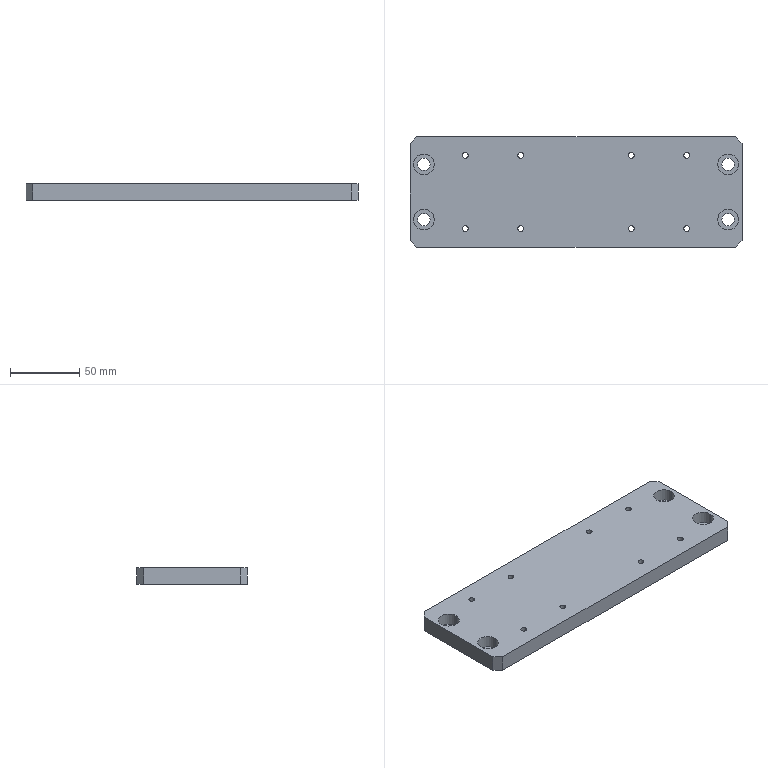Part | SolidWorks | features BaseBody 1 | 1 solid | 46 faces | box 240 x 80 x 12 mm | volume 221345 mm3 | cylinder 32 | plane 14 | commonest cylinder face diameters 4.2 x16 9 x8 15 x8
STEP:
#1=CARTESIAN_POINT('',(77.9,26.5,0.));
#2=VERTEX_POINT('',#1);
#3=CARTESIAN_POINT('',(82.1,26.5,0.));
#4=VERTEX_POINT('',#3);
#5=CARTESIAN_POINT('',(80.,26.5,0.));
#6=DIRECTION('',(0.,0.,1.));
#7=DIRECTION('',(1.,0.,0.));
#8=AXIS2_PLACEMENT_3D('',#5,#6,#7);
#9=CIRCLE('',#8,2.1);
#10=EDGE_CURVE('',#2,#4,#9,.T.);
#11=ORIENTED_EDGE('',*,*,#10,.F.);
#12=CARTESIAN_POINT('',(77.9,26.5,12.));
#13=VERTEX_POINT('',#12);
#14=CARTESIAN_POINT('',(77.9,26.5,12.));
#15=DIRECTION('',(0.,0.,1.));
#16=VECTOR('',#15,1000.);
#17=LINE('',#14,#16);
#18=EDGE_CURVE('',#2,#13,#17,.T.);
#19=ORIENTED_EDGE('',*,*,#18,.T.);
#20=CARTESIAN_POINT('',(82.1,26.5,12.));
#21=VERTEX_POINT('',#20);
#22=CARTESIAN_POINT('',(80.,26.5,12.));
#23=DIRECTION('',(0.,0.,-1.));
#24=DIRECTION('',(1.,0.,0.));
#25=AXIS2_PLACEMENT_3D('',#22,#23,#24);
#26=CIRCLE('',#25,2.1);
#27=EDGE_CURVE('',#21,#13,#26,.T.);
#28=ORIENTED_EDGE('',*,*,#27,.F.);
#29=CARTESIAN_POINT('',(82.1,26.5,12.));
#30=DIRECTION('',(0.,0.,1.));
#31=VECTOR('',#30,1000.);
#32=LINE('',#29,#31);
#33=EDGE_CURVE('',#4,#21,#32,.T.);
#34=ORIENTED_EDGE('',*,*,#33,.F.);
#35=EDGE_LOOP('',(#11,#19,#28,#34));
#36=FACE_OUTER_BOUND('',#35,.T.);
#37=CARTESIAN_POINT('',(80.,26.5,12.));
#38=DIRECTION('',(0.,0.,1.));
#39=DIRECTION('',(1.,0.,0.));
#40=AXIS2_PLACEMENT_3D('',#37,#38,#39);
#41=CYLINDRICAL_SURFACE('',#40,2.1);
#42=ADVANCED_FACE('',(#36),#41,.F.);
#43=CARTESIAN_POINT('',(77.9,-26.5,0.));
#44=VERTEX_POINT('',#43);
#45=CARTESIAN_POINT('',(82.1,-26.5,0.));
#46=VERTEX_POINT('',#45);
#47=CARTESIAN_POINT('',(80.,-26.5,0.));
#48=DIRECTION('',(0.,0.,1.));
#49=DIRECTION('',(1.,0.,0.));
#50=AXIS2_PLACEMENT_3D('',#47,#48,#49);
#51=CIRCLE('',#50,2.1);
#52=EDGE_CURVE('',#44,#46,#51,.T.);
#53=ORIENTED_EDGE('',*,*,#52,.F.);
#54=CARTESIAN_POINT('',(77.9,-26.5,12.));
#55=VERTEX_POINT('',#54);
#56=CARTESIAN_POINT('',(77.9,-26.5,12.));
#57=DIRECTION('',(0.,0.,1.));
#58=VECTOR('',#57,1000.);
#59=LINE('',#56,#58);
#60=EDGE_CURVE('',#44,#55,#59,.T.);
#61=ORIENTED_EDGE('',*,*,#60,.T.);
#62=CARTESIAN_POINT('',(82.1,-26.5,12.));
#63=VERTEX_POINT('',#62);
#64=CARTESIAN_POINT('',(80.,-26.5,12.));
#65=DIRECTION('',(0.,0.,-1.));
#66=DIRECTION('',(1.,0.,0.));
#67=AXIS2_PLACEMENT_3D('',#64,#65,#66);
#68=CIRCLE('',#67,2.1);
#69=EDGE_CURVE('',#63,#55,#68,.T.);
#70=ORIENTED_EDGE('',*,*,#69,.F.);
#71=CARTESIAN_POINT('',(82.1,-26.5,12.));
#72=DIRECTION('',(0.,0.,1.));
#73=VECTOR('',#72,1000.);
#74=LINE('',#71,#73);
#75=EDGE_CURVE('',#46,#63,#74,.T.);
#76=ORIENTED_EDGE('',*,*,#75,.F.);
#77=EDGE_LOOP('',(#53,#61,#70,#76));
#78=FACE_OUTER_BOUND('',#77,.T.);
#79=CARTESIAN_POINT('',(80.,-26.5,12.));
#80=DIRECTION('',(0.,0.,1.));
#81=DIRECTION('',(1.,0.,0.));
#82=AXIS2_PLACEMENT_3D('',#79,#80,#81);
#83=CYLINDRICAL_SURFACE('',#82,2.1);
#84=ADVANCED_FACE('',(#78),#83,.F.);
#85=CARTESIAN_POINT('',(37.9,-26.5,0.));
#86=VERTEX_POINT('',#85);
#87=CARTESIAN_POINT('',(42.1,-26.5,0.));
#88=VERTEX_POINT('',#87);
#89=CARTESIAN_POINT('',(40.,-26.5,0.));
#90=DIRECTION('',(0.,0.,1.));
#91=DIRECTION('',(1.,0.,0.));
#92=AXIS2_PLACEMENT_3D('',#89,#90,#91);
#93=CIRCLE('',#92,2.1);
#94=EDGE_CURVE('',#86,#88,#93,.T.);
#95=ORIENTED_EDGE('',*,*,#94,.F.);
#96=CARTESIAN_POINT('',(37.9,-26.5,12.));
#97=VERTEX_POINT('',#96);
#98=CARTESIAN_POINT('',(37.9,-26.5,12.));
#99=DIRECTION('',(0.,0.,1.));
#100=VECTOR('',#99,1000.);
#101=LINE('',#98,#100);
#102=EDGE_CURVE('',#86,#97,#101,.T.);
#103=ORIENTED_EDGE('',*,*,#102,.T.);
#104=CARTESIAN_POINT('',(42.1,-26.5,12.));
#105=VERTEX_POINT('',#104);
#106=CARTESIAN_POINT('',(40.,-26.5,12.));
#107=DIRECTION('',(0.,0.,-1.));
#108=DIRECTION('',(1.,0.,0.));
#109=AXIS2_PLACEMENT_3D('',#106,#107,#108);
#110=CIRCLE('',#109,2.1);
#111=EDGE_CURVE('',#105,#97,#110,.T.);
#112=ORIENTED_EDGE('',*,*,#111,.F.);
#113=CARTESIAN_POINT('',(42.1,-26.5,12.));
#114=DIRECTION('',(0.,0.,1.));
#115=VECTOR('',#114,1000.);
#116=LINE('',#113,#115);
#117=EDGE_CURVE('',#88,#105,#116,.T.);
#118=ORIENTED_EDGE('',*,*,#117,.F.);
#119=EDGE_LOOP('',(#95,#103,#112,#118));
#120=FACE_OUTER_BOUND('',#119,.T.);
#121=CARTESIAN_POINT('',(40.,-26.5,12.));
#122=DIRECTION('',(0.,0.,1.));
#123=DIRECTION('',(1.,0.,0.));
#124=AXIS2_PLACEMENT_3D('',#121,#122,#123);
#125=CYLINDRICAL_SURFACE('',#124,2.1);
#126=ADVANCED_FACE('',(#120),#125,.F.);
#127=CARTESIAN_POINT('',(37.9,26.5,0.));
#128=VERTEX_POINT('',#127);
#129=CARTESIAN_POINT('',(42.1,26.5,0.));
#130=VERTEX_POINT('',#129);
#131=CARTESIAN_POINT('',(40.,26.5,0.));
#132=DIRECTION('',(0.,0.,1.));
#133=DIRECTION('',(1.,0.,0.));
#134=AXIS2_PLACEMENT_3D('',#131,#132,#133);
#135=CIRCLE('',#134,2.1);
#136=EDGE_CURVE('',#128,#130,#135,.T.);
#137=ORIENTED_EDGE('',*,*,#136,.F.);
#138=CARTESIAN_POINT('',(37.9,26.5,12.));
#139=VERTEX_POINT('',#138);
#140=CARTESIAN_POINT('',(37.9,26.5,12.));
#141=DIRECTION('',(0.,0.,1.));
#142=VECTOR('',#141,1000.);
#143=LINE('',#140,#142);
#144=EDGE_CURVE('',#128,#139,#143,.T.);
#145=ORIENTED_EDGE('',*,*,#144,.T.);
#146=CARTESIAN_POINT('',(42.1,26.5,12.));
#147=VERTEX_POINT('',#146);
#148=CARTESIAN_POINT('',(40.,26.5,12.));
#149=DIRECTION('',(0.,0.,-1.));
#150=DIRECTION('',(1.,0.,0.));
#151=AXIS2_PLACEMENT_3D('',#148,#149,#150);
#152=CIRCLE('',#151,2.1);
#153=EDGE_CURVE('',#147,#139,#152,.T.);
#154=ORIENTED_EDGE('',*,*,#153,.F.);
#155=CARTESIAN_POINT('',(42.1,26.5,12.));
#156=DIRECTION('',(0.,0.,1.));
#157=VECTOR('',#156,1000.);
#158=LINE('',#155,#157);
#159=EDGE_CURVE('',#130,#147,#158,.T.);
#160=ORIENTED_EDGE('',*,*,#159,.F.);
#161=EDGE_LOOP('',(#137,#145,#154,#160));
#162=FACE_OUTER_BOUND('',#161,.T.);
#163=CARTESIAN_POINT('',(40.,26.5,12.));
#164=DIRECTION('',(0.,0.,1.));
#165=DIRECTION('',(1.,0.,0.));
#166=AXIS2_PLACEMENT_3D('',#163,#164,#165);
#167=CYLINDRICAL_SURFACE('',#166,2.1);
#168=ADVANCED_FACE('',(#162),#167,.F.);
#169=CARTESIAN_POINT('',(-42.1,26.5,0.));
#170=VERTEX_POINT('',#169);
#171=CARTESIAN_POINT('',(-37.9,26.5,0.));
#172=VERTEX_POINT('',#171);
#173=CARTESIAN_POINT('',(-40.,26.5,0.));
#174=DIRECTION('',(0.,0.,1.));
#175=DIRECTION('',(1.,0.,0.));
#176=AXIS2_PLACEMENT_3D('',#173,#174,#175);
#177=CIRCLE('',#176,2.1);
#178=EDGE_CURVE('',#170,#172,#177,.T.);
#179=ORIENTED_EDGE('',*,*,#178,.F.);
#180=CARTESIAN_POINT('',(-42.1,26.5,12.));
#181=VERTEX_POINT('',#180);
#182=CARTESIAN_POINT('',(-42.1,26.5,12.));
#183=DIRECTION('',(0.,0.,1.));
#184=VECTOR('',#183,1000.);
#185=LINE('',#182,#184);
#186=EDGE_CURVE('',#170,#181,#185,.T.);
#187=ORIENTED_EDGE('',*,*,#186,.T.);
#188=CARTESIAN_POINT('',(-37.9,26.5,12.));
#189=VERTEX_POINT('',#188);
#190=CARTESIAN_POINT('',(-40.,26.5,12.));
#191=DIRECTION('',(0.,0.,-1.));
#192=DIRECTION('',(1.,0.,0.));
#193=AXIS2_PLACEMENT_3D('',#190,#191,#192);
#194=CIRCLE('',#193,2.1);
#195=EDGE_CURVE('',#189,#181,#194,.T.);
#196=ORIENTED_EDGE('',*,*,#195,.F.);
#197=CARTESIAN_POINT('',(-37.9,26.5,12.));
#198=DIRECTION('',(0.,0.,1.));
#199=VECTOR('',#198,1000.);
#200=LINE('',#197,#199);
#201=EDGE_CURVE('',#172,#189,#200,.T.);
#202=ORIENTED_EDGE('',*,*,#201,.F.);
#203=EDGE_LOOP('',(#179,#187,#196,#202));
#204=FACE_OUTER_BOUND('',#203,.T.);
#205=CARTESIAN_POINT('',(-40.,26.5,12.));
#206=DIRECTION('',(0.,0.,1.));
#207=DIRECTION('',(1.,0.,0.));
#208=AXIS2_PLACEMENT_3D('',#205,#206,#207);
#209=CYLINDRICAL_SURFACE('',#208,2.1);
#210=ADVANCED_FACE('',(#204),#209,.F.);
#211=CARTESIAN_POINT('',(-42.1,-26.5,0.));
#212=VERTEX_POINT('',#211);
#213=CARTESIAN_POINT('',(-37.9,-26.5,0.));
#214=VERTEX_POINT('',#213);
#215=CARTESIAN_POINT('',(-40.,-26.5,0.));
#216=DIRECTION('',(0.,0.,1.));
#217=DIRECTION('',(1.,0.,0.));
#218=AXIS2_PLACEMENT_3D('',#215,#216,#217);
#219=CIRCLE('',#218,2.1);
#220=EDGE_CURVE('',#212,#214,#219,.T.);
#221=ORIENTED_EDGE('',*,*,#220,.F.);
#222=CARTESIAN_POINT('',(-42.1,-26.5,12.));
#223=VERTEX_POINT('',#222);
#224=CARTESIAN_POINT('',(-42.1,-26.5,12.));
#225=DIRECTION('',(0.,0.,1.));
#226=VECTOR('',#225,1000.);
#227=LINE('',#224,#226);
#228=EDGE_CURVE('',#212,#223,#227,.T.);
#229=ORIENTED_EDGE('',*,*,#228,.T.);
#230=CARTESIAN_POINT('',(-37.9,-26.5,12.));
#231=VERTEX_POINT('',#230);
#232=CARTESIAN_POINT('',(-40.,-26.5,12.));
#233=DIRECTION('',(0.,0.,-1.));
#234=DIRECTION('',(1.,0.,0.));
#235=AXIS2_PLACEMENT_3D('',#232,#233,#234);
#236=CIRCLE('',#235,2.1);
#237=EDGE_CURVE('',#231,#223,#236,.T.);
#238=ORIENTED_EDGE('',*,*,#237,.F.);
#239=CARTESIAN_POINT('',(-37.9,-26.5,12.));
#240=DIRECTION('',(0.,0.,1.));
#241=VECTOR('',#240,1000.);
#242=LINE('',#239,#241);
#243=EDGE_CURVE('',#214,#231,#242,.T.);
#244=ORIENTED_EDGE('',*,*,#243,.F.);
#245=EDGE_LOOP('',(#221,#229,#238,#244));
#246=FACE_OUTER_BOUND('',#245,.T.);
#247=CARTESIAN_POINT('',(-40.,-26.5,12.));
#248=DIRECTION('',(0.,0.,1.));
#249=DIRECTION('',(1.,0.,0.));
#250=AXIS2_PLACEMENT_3D('',#247,#248,#249);
#251=CYLINDRICAL_SURFACE('',#250,2.1);
#252=ADVANCED_FACE('',(#246),#251,.F.);
#253=CARTESIAN_POINT('',(-82.1,-26.5,0.));
#254=VERTEX_POINT('',#253);
#255=CARTESIAN_POINT('',(-77.9,-26.5,0.));
#256=VERTEX_POINT('',#255);
#257=CARTESIAN_POINT('',(-80.,-26.5,0.));
#258=DIRECTION('',(0.,0.,1.));
#259=DIRECTION('',(1.,0.,0.));
#260=AXIS2_PLACEMENT_3D('',#257,#258,#259);
#261=CIRCLE('',#260,2.1);
#262=EDGE_CURVE('',#254,#256,#261,.T.);
#263=ORIENTED_EDGE('',*,*,#262,.F.);
#264=CARTESIAN_POINT('',(-82.1,-26.5,12.));
#265=VERTEX_POINT('',#264);
#266=CARTESIAN_POINT('',(-82.1,-26.5,12.));
#267=DIRECTION('',(0.,0.,1.));
#268=VECTOR('',#267,1000.);
#269=LINE('',#266,#268);
#270=EDGE_CURVE('',#254,#265,#269,.T.);
#271=ORIENTED_EDGE('',*,*,#270,.T.);
#272=CARTESIAN_POINT('',(-77.9,-26.5,12.));
#273=VERTEX_POINT('',#272);
#274=CARTESIAN_POINT('',(-80.,-26.5,12.));
#275=DIRECTION('',(0.,0.,-1.));
#276=DIRECTION('',(1.,0.,0.));
#277=AXIS2_PLACEMENT_3D('',#274,#275,#276);
#278=CIRCLE('',#277,2.1);
#279=EDGE_CURVE('',#273,#265,#278,.T.);
#280=ORIENTED_EDGE('',*,*,#279,.F.);
#281=CARTESIAN_POINT('',(-77.9,-26.5,12.));
#282=DIRECTION('',(0.,0.,1.));
#283=VECTOR('',#282,1000.);
#284=LINE('',#281,#283);
#285=EDGE_CURVE('',#256,#273,#284,.T.);
#286=ORIENTED_EDGE('',*,*,#285,.F.);
#287=EDGE_LOOP('',(#263,#271,#280,#286));
#288=FACE_OUTER_BOUND('',#287,.T.);
#289=CARTESIAN_POINT('',(-80.,-26.5,12.));
#290=DIRECTION('',(0.,0.,1.));
#291=DIRECTION('',(1.,0.,0.));
#292=AXIS2_PLACEMENT_3D('',#289,#290,#291);
#293=CYLINDRICAL_SURFACE('',#292,2.1);
#294=ADVANCED_FACE('',(#288),#293,.F.);
#295=CARTESIAN_POINT('',(-82.1,26.5,0.));
#296=VERTEX_POINT('',#295);
#297=CARTESIAN_POINT('',(-77.9,26.5,0.));
#298=VERTEX_POINT('',#297);
#299=CARTESIAN_POINT('',(-80.,26.5,0.));
#300=DIRECTION('',(0.,0.,1.));
#301=DIRECTION('',(1.,0.,0.));
#302=AXIS2_PLACEMENT_3D('',#299,#300,#301);
#303=CIRCLE('',#302,2.1);
#304=EDGE_CURVE('',#296,#298,#303,.T.);
#305=ORIENTED_EDGE('',*,*,#304,.F.);
#306=CARTESIAN_POINT('',(-82.1,26.5,12.));
#307=VERTEX_POINT('',#306);
#308=CARTESIAN_POINT('',(-82.1,26.5,12.));
#309=DIRECTION('',(0.,0.,1.));
#310=VECTOR('',#309,1000.);
#311=LINE('',#308,#310);
#312=EDGE_CURVE('',#296,#307,#311,.T.);
#313=ORIENTED_EDGE('',*,*,#312,.T.);
#314=CARTESIAN_POINT('',(-77.9,26.5,12.));
#315=VERTEX_POINT('',#314);
#316=CARTESIAN_POINT('',(-80.,26.5,12.));
#317=DIRECTION('',(0.,0.,-1.));
#318=DIRECTION('',(1.,0.,0.));
#319=AXIS2_PLACEMENT_3D('',#316,#317,#318);
#320=CIRCLE('',#319,2.1);
#321=EDGE_CURVE('',#315,#307,#320,.T.);
#322=ORIENTED_EDGE('',*,*,#321,.F.);
#323=CARTESIAN_POINT('',(-77.9,26.5,12.));
#324=DIRECTION('',(0.,0.,1.));
#325=VECTOR('',#324,1000.);
#326=LINE('',#323,#325);
#327=EDGE_CURVE('',#298,#315,#326,.T.);
#328=ORIENTED_EDGE('',*,*,#327,.F.);
#329=EDGE_LOOP('',(#305,#313,#322,#328));
#330=FACE_OUTER_BOUND('',#329,.T.);
#331=CARTESIAN_POINT('',(-80.,26.5,12.));
#332=DIRECTION('',(0.,0.,1.));
#333=DIRECTION('',(1.,0.,0.));
#334=AXIS2_PLACEMENT_3D('',#331,#332,#333);
#335=CYLINDRICAL_SURFACE('',#334,2.1);
#336=ADVANCED_FACE('',(#330),#335,.F.);
#337=CARTESIAN_POINT('',(105.5,20.,0.));
#338=VERTEX_POINT('',#337);
#339=CARTESIAN_POINT('',(114.5,20.,0.));
#340=VERTEX_POINT('',#339);
#341=CARTESIAN_POINT('',(110.,20.,0.));
#342=DIRECTION('',(0.,0.,1.));
#343=DIRECTION('',(1.,0.,0.));
#344=AXIS2_PLACEMENT_3D('',#341,#342,#343);
#345=CIRCLE('',#344,4.5);
#346=EDGE_CURVE('',#338,#340,#345,.T.);
#347=ORIENTED_EDGE('',*,*,#346,.F.);
#348=CARTESIAN_POINT('',(105.5,20.,3.));
#349=VERTEX_POINT('',#348);
#350=CARTESIAN_POINT('',(105.5,20.,12.));
#351=DIRECTION('',(0.,0.,1.));
#352=VECTOR('',#351,1000.);
#353=LINE('',#350,#352);
#354=EDGE_CURVE('',#338,#349,#353,.T.);
#355=ORIENTED_EDGE('',*,*,#354,.T.);
#356=CARTESIAN_POINT('',(114.5,20.,3.));
#357=VERTEX_POINT('',#356);
#358=CARTESIAN_POINT('',(110.,20.,3.));
#359=DIRECTION('',(0.,0.,-1.));
#360=DIRECTION('',(1.,0.,0.));
#361=AXIS2_PLACEMENT_3D('',#358,#359,#360);
#362=CIRCLE('',#361,4.5);
#363=EDGE_CURVE('',#357,#349,#362,.T.);
#364=ORIENTED_EDGE('',*,*,#363,.F.);
#365=CARTESIAN_POINT('',(114.5,20.,12.));
#366=DIRECTION('',(0.,0.,1.));
#367=VECTOR('',#366,1000.);
#368=LINE('',#365,#367);
#369=EDGE_CURVE('',#340,#357,#368,.T.);
#370=ORIENTED_EDGE('',*,*,#369,.F.);
#371=EDGE_LOOP('',(#347,#355,#364,#370));
#372=FACE_OUTER_BOUND('',#371,.T.);
#373=CARTESIAN_POINT('',(110.,20.,12.));
#374=DIRECTION('',(0.,0.,1.));
#375=DIRECTION('',(1.,0.,0.));
#376=AXIS2_PLACEMENT_3D('',#373,#374,#375);
#377=CYLINDRICAL_SURFACE('',#376,4.5);
#378=ADVANCED_FACE('',(#372),#377,.F.);
#379=CARTESIAN_POINT('',(105.5,-20.,0.));
#380=VERTEX_POINT('',#379);
#381=CARTESIAN_POINT('',(114.5,-20.,0.));
#382=VERTEX_POINT('',#381);
#383=CARTESIAN_POINT('',(110.,-20.,0.));
#384=DIRECTION('',(0.,0.,1.));
#385=DIRECTION('',(1.,0.,0.));
#386=AXIS2_PLACEMENT_3D('',#383,#384,#385);
#387=CIRCLE('',#386,4.5);
#388=EDGE_CURVE('',#380,#382,#387,.T.);
#389=ORIENTED_EDGE('',*,*,#388,.F.);
#390=CARTESIAN_POINT('',(105.5,-20.,3.));
#391=VERTEX_POINT('',#390);
#392=CARTESIAN_POINT('',(105.5,-20.,12.));
#393=DIRECTION('',(0.,0.,1.));
#394=VECTOR('',#393,1000.);
#395=LINE('',#392,#394);
#396=EDGE_CURVE('',#380,#391,#395,.T.);
#397=ORIENTED_EDGE('',*,*,#396,.T.);
#398=CARTESIAN_POINT('',(114.5,-20.,3.));
#399=VERTEX_POINT('',#398);
#400=CARTESIAN_POINT('',(110.,-20.,3.));
#401=DIRECTION('',(0.,0.,-1.));
#402=DIRECTION('',(1.,0.,0.));
#403=AXIS2_PLACEMENT_3D('',#400,#401,#402);
#404=CIRCLE('',#403,4.5);
#405=EDGE_CURVE('',#399,#391,#404,.T.);
#406=ORIENTED_EDGE('',*,*,#405,.F.);
#407=CARTESIAN_POINT('',(114.5,-20.,12.));
#408=DIRECTION('',(0.,0.,1.));
#409=VECTOR('',#408,1000.);
#410=LINE('',#407,#409);
#411=EDGE_CURVE('',#382,#399,#410,.T.);
#412=ORIENTED_EDGE('',*,*,#411,.F.);
#413=EDGE_LOOP('',(#389,#397,#406,#412));
#414=FACE_OUTER_BOUND('',#413,.T.);
#415=CARTESIAN_POINT('',(110.,-20.,12.));
#416=DIRECTION('',(0.,0.,1.));
#417=DIRECTION('',(1.,0.,0.));
#418=AXIS2_PLACEMENT_3D('',#415,#416,#417);
#419=CYLINDRICAL_SURFACE('',#418,4.5);
#420=ADVANCED_FACE('',(#414),#419,.F.);
#421=CARTESIAN_POINT('',(-114.5,-20.,0.));
#422=VERTEX_POINT('',#421);
#423=CARTESIAN_POINT('',(-105.5,-20.,0.));
#424=VERTEX_POINT('',#423);
#425=CARTESIAN_POINT('',(-110.,-20.,0.));
#426=DIRECTION('',(0.,0.,1.));
#427=DIRECTION('',(1.,0.,0.));
#428=AXIS2_PLACEMENT_3D('',#425,#426,#427);
#429=CIRCLE('',#428,4.5);
#430=EDGE_CURVE('',#422,#424,#429,.T.);
#431=ORIENTED_EDGE('',*,*,#430,.F.);
#432=CARTESIAN_POINT('',(-114.5,-20.,3.));
#433=VERTEX_POINT('',#432);
#434=CARTESIAN_POINT('',(-114.5,-20.,12.));
#435=DIRECTION('',(0.,0.,1.));
#436=VECTOR('',#435,1000.);
#437=LINE('',#434,#436);
#438=EDGE_CURVE('',#422,#433,#437,.T.);
#439=ORIENTED_EDGE('',*,*,#438,.T.);
#440=CARTESIAN_POINT('',(-105.5,-20.,3.));
#441=VERTEX_POINT('',#440);
#442=CARTESIAN_POINT('',(-110.,-20.,3.));
#443=DIRECTION('',(0.,0.,-1.));
#444=DIRECTION('',(1.,0.,0.));
#445=AXIS2_PLACEMENT_3D('',#442,#443,#444);
#446=CIRCLE('',#445,4.5);
#447=EDGE_CURVE('',#441,#433,#446,.T.);
#448=ORIENTED_EDGE('',*,*,#447,.F.);
#449=CARTESIAN_POINT('',(-105.5,-20.,12.));
#450=DIRECTION('',(0.,0.,1.));
#451=VECTOR('',#450,1000.);
#452=LINE('',#449,#451);
#453=EDGE_CURVE('',#424,#441,#452,.T.);
#454=ORIENTED_EDGE('',*,*,#453,.F.);
#455=EDGE_LOOP('',(#431,#439,#448,#454));
#456=FACE_OUTER_BOUND('',#455,.T.);
#457=CARTESIAN_POINT('',(-110.,-20.,12.));
#458=DIRECTION('',(0.,0.,1.));
#459=DIRECTION('',(1.,0.,0.));
#460=AXIS2_PLACEMENT_3D('',#457,#458,#459);
#461=CYLINDRICAL_SURFACE('',#460,4.5);
#462=ADVANCED_FACE('',(#456),#461,.F.);
#463=CARTESIAN_POINT('',(-114.5,20.,0.));
#464=VERTEX_POINT('',#463);
#465=CARTESIAN_POINT('',(-105.5,20.,0.));
#466=VERTEX_POINT('',#465);
#467=CARTESIAN_POINT('',(-110.,20.,0.));
#468=DIRECTION('',(0.,0.,1.));
#469=DIRECTION('',(1.,0.,0.));
#470=AXIS2_PLACEMENT_3D('',#467,#468,#469);
#471=CIRCLE('',#470,4.5);
#472=EDGE_CURVE('',#464,#466,#471,.T.);
#473=ORIENTED_EDGE('',*,*,#472,.F.);
#474=CARTESIAN_POINT('',(-114.5,20.,3.));
#475=VERTEX_POINT('',#474);
#476=CARTESIAN_POINT('',(-114.5,20.,12.));
#477=DIRECTION('',(0.,0.,1.));
#478=VECTOR('',#477,1000.);
#479=LINE('',#476,#478);
#480=EDGE_CURVE('',#464,#475,#479,.T.);
#481=ORIENTED_EDGE('',*,*,#480,.T.);
#482=CARTESIAN_POINT('',(-105.5,20.,3.));
#483=VERTEX_POINT('',#482);
#484=CARTESIAN_POINT('',(-110.,20.,3.));
#485=DIRECTION('',(0.,0.,-1.));
#486=DIRECTION('',(1.,0.,0.));
#487=AXIS2_PLACEMENT_3D('',#484,#485,#486);
#488=CIRCLE('',#487,4.5);
#489=EDGE_CURVE('',#483,#475,#488,.T.);
#490=ORIENTED_EDGE('',*,*,#489,.F.);
#491=CARTESIAN_POINT('',(-105.5,20.,12.));
#492=DIRECTION('',(0.,0.,1.));
#493=VECTOR('',#492,1000.);
#494=LINE('',#491,#493);
#495=EDGE_CURVE('',#466,#483,#494,.T.);
#496=ORIENTED_EDGE('',*,*,#495,.F.);
#497=EDGE_LOOP('',(#473,#481,#490,#496));
#498=FACE_OUTER_BOUND('',#497,.T.);
#499=CARTESIAN_POINT('',(-110.,20.,12.));
#500=DIRECTION('',(0.,0.,1.));
#501=DIRECTION('',(1.,0.,0.));
#502=AXIS2_PLACEMENT_3D('',#499,#500,#501);
#503=CYLINDRICAL_SURFACE('',#502,4.5);
#504=ADVANCED_FACE('',(#498),#503,.F.);
#505=CARTESIAN_POINT('',(-102.5,-20.,3.));
#506=VERTEX_POINT('',#505);
#507=CARTESIAN_POINT('',(-117.5,-20.,3.));
#508=VERTEX_POINT('',#507);
#509=CARTESIAN_POINT('',(-110.,-20.,3.));
#510=DIRECTION('',(0.,0.,-1.));
#511=DIRECTION('',(1.,0.,0.));
#512=AXIS2_PLACEMENT_3D('',#509,#510,#511);
#513=CIRCLE('',#512,7.5);
#514=EDGE_CURVE('',#506,#508,#513,.T.);
#515=ORIENTED_EDGE('',*,*,#514,.T.);
#516=CARTESIAN_POINT('',(-117.5,-20.,12.));
#517=VERTEX_POINT('',#516);
#518=CARTESIAN_POINT('',(-117.5,-20.,12.));
#519=DIRECTION('',(0.,0.,1.));
#520=VECTOR('',#519,1000.);
#521=LINE('',#518,#520);
#522=EDGE_CURVE('',#508,#517,#521,.T.);
#523=ORIENTED_EDGE('',*,*,#522,.T.);
#524=CARTESIAN_POINT('',(-102.5,-20.,12.));
#525=VERTEX_POINT('',#524);
#526=CARTESIAN_POINT('',(-110.,-20.,12.));
#527=DIRECTION('',(0.,0.,1.));
#528=DIRECTION('',(1.,0.,0.));
#529=AXIS2_PLACEMENT_3D('',#526,#527,#528);
#530=CIRCLE('',#529,7.5);
#531=EDGE_CURVE('',#517,#525,#530,.T.);
#532=ORIENTED_EDGE('',*,*,#531,.T.);
#533=CARTESIAN_POINT('',(-102.5,-20.,12.));
#534=DIRECTION('',(0.,0.,1.));
#535=VECTOR('',#534,1000.);
#536=LINE('',#533,#535);
#537=EDGE_CURVE('',#506,#525,#536,.T.);
#538=ORIENTED_EDGE('',*,*,#537,.F.);
#539=EDGE_LOOP('',(#515,#523,#532,#538));
#540=FACE_OUTER_BOUND('',#539,.T.);
#541=CARTESIAN_POINT('',(-110.,-20.,12.));
#542=DIRECTION('',(0.,0.,1.));
#543=DIRECTION('',(1.,0.,0.));
#544=AXIS2_PLACEMENT_3D('',#541,#542,#543);
#545=CYLINDRICAL_SURFACE('',#544,7.5);
#546=ADVANCED_FACE('',(#540),#545,.F.);
#547=CARTESIAN_POINT('',(117.5,-20.,3.));
#548=VERTEX_POINT('',#547);
#549=CARTESIAN_POINT('',(102.5,-20.,3.));
#550=VERTEX_POINT('',#549);
#551=CARTESIAN_POINT('',(110.,-20.,3.));
#552=DIRECTION('',(0.,0.,-1.));
#553=DIRECTION('',(1.,0.,0.));
#554=AXIS2_PLACEMENT_3D('',#551,#552,#553);
#555=CIRCLE('',#554,7.5);
#556=EDGE_CURVE('',#548,#550,#555,.T.);
#557=ORIENTED_EDGE('',*,*,#556,.T.);
#558=CARTESIAN_POINT('',(102.5,-20.,12.));
#559=VERTEX_POINT('',#558);
#560=CARTESIAN_POINT('',(102.5,-20.,12.));
#561=DIRECTION('',(0.,0.,1.));
#562=VECTOR('',#561,1000.);
#563=LINE('',#560,#562);
#564=EDGE_CURVE('',#550,#559,#563,.T.);
#565=ORIENTED_EDGE('',*,*,#564,.T.);
#566=CARTESIAN_POINT('',(117.5,-20.,12.));
#567=VERTEX_POINT('',#566);
#568=CARTESIAN_POINT('',(110.,-20.,12.));
#569=DIRECTION('',(0.,0.,1.));
#570=DIRECTION('',(1.,0.,0.));
#571=AXIS2_PLACEMENT_3D('',#568,#569,#570);
#572=CIRCLE('',#571,7.5);
#573=EDGE_CURVE('',#559,#567,#572,.T.);
#574=ORIENTED_EDGE('',*,*,#573,.T.);
#575=CARTESIAN_POINT('',(117.5,-20.,12.));
#576=DIRECTION('',(0.,0.,1.));
#577=VECTOR('',#576,1000.);
#578=LINE('',#575,#577);
#579=EDGE_CURVE('',#548,#567,#578,.T.);
#580=ORIENTED_EDGE('',*,*,#579,.F.);
#581=EDGE_LOOP('',(#557,#565,#574,#580));
#582=FACE_OUTER_BOUND('',#581,.T.);
#583=CARTESIAN_POINT('',(110.,-20.,12.));
#584=DIRECTION('',(0.,0.,1.));
#585=DIRECTION('',(1.,0.,0.));
#586=AXIS2_PLACEMENT_3D('',#583,#584,#585);
#587=CYLINDRICAL_SURFACE('',#586,7.5);
#588=ADVANCED_FACE('',(#582),#587,.F.);
#589=CARTESIAN_POINT('',(117.5,20.,3.));
#590=VERTEX_POINT('',#589);
#591=CARTESIAN_POINT('',(102.5,20.,3.));
#592=VERTEX_POINT('',#591);
#593=CARTESIAN_POINT('',(110.,20.,3.));
#594=DIRECTION('',(0.,0.,-1.));
#595=DIRECTION('',(1.,0.,0.));
#596=AXIS2_PLACEMENT_3D('',#593,#594,#595);
#597=CIRCLE('',#596,7.5);
#598=EDGE_CURVE('',#590,#592,#597,.T.);
#599=ORIENTED_EDGE('',*,*,#598,.T.);
#600=CARTESIAN_POINT('',(102.5,20.,12.));
#601=VERTEX_POINT('',#600);
#602=CARTESIAN_POINT('',(102.5,20.,12.));
#603=DIRECTION('',(0.,0.,1.));
#604=VECTOR('',#603,1000.);
#605=LINE('',#602,#604);
#606=EDGE_CURVE('',#592,#601,#605,.T.);
#607=ORIENTED_EDGE('',*,*,#606,.T.);
#608=CARTESIAN_POINT('',(117.5,20.,12.));
#609=VERTEX_POINT('',#608);
#610=CARTESIAN_POINT('',(110.,20.,12.));
#611=DIRECTION('',(0.,0.,1.));
#612=DIRECTION('',(1.,0.,0.));
#613=AXIS2_PLACEMENT_3D('',#610,#611,#612);
#614=CIRCLE('',#613,7.5);
#615=EDGE_CURVE('',#601,#609,#614,.T.);
#616=ORIENTED_EDGE('',*,*,#615,.T.);
#617=CARTESIAN_POINT('',(117.5,20.,12.));
#618=DIRECTION('',(0.,0.,1.));
#619=VECTOR('',#618,1000.);
#620=LINE('',#617,#619);
#621=EDGE_CURVE('',#590,#609,#620,.T.);
#622=ORIENTED_EDGE('',*,*,#621,.F.);
#623=EDGE_LOOP('',(#599,#607,#616,#622));
#624=FACE_OUTER_BOUND('',#623,.T.);
#625=CARTESIAN_POINT('',(110.,20.,12.));
#626=DIRECTION('',(0.,0.,1.));
#627=DIRECTION('',(1.,0.,0.));
#628=AXIS2_PLACEMENT_3D('',#625,#626,#627);
#629=CYLINDRICAL_SURFACE('',#628,7.5);
#630=ADVANCED_FACE('',(#624),#629,.F.);
#631=CARTESIAN_POINT('',(-102.5,20.,3.));
#632=VERTEX_POINT('',#631);
#633=CARTESIAN_POINT('',(-117.5,20.,3.));
#634=VERTEX_POINT('',#633);
#635=CARTESIAN_POINT('',(-110.,20.,3.));
#636=DIRECTION('',(0.,0.,-1.));
#637=DIRECTION('',(1.,0.,0.));
#638=AXIS2_PLACEMENT_3D('',#635,#636,#637);
#639=CIRCLE('',#638,7.5);
#640=EDGE_CURVE('',#632,#634,#639,.T.);
#641=ORIENTED_EDGE('',*,*,#640,.T.);
#642=CARTESIAN_POINT('',(-117.5,20.,12.));
#643=VERTEX_POINT('',#642);
#644=CARTESIAN_POINT('',(-117.5,20.,12.));
#645=DIRECTION('',(0.,0.,1.));
#646=VECTOR('',#645,1000.);
#647=LINE('',#644,#646);
#648=EDGE_CURVE('',#634,#643,#647,.T.);
#649=ORIENTED_EDGE('',*,*,#648,.T.);
#650=CARTESIAN_POINT('',(-102.5,20.,12.));
#651=VERTEX_POINT('',#650);
#652=CARTESIAN_POINT('',(-110.,20.,12.));
#653=DIRECTION('',(0.,0.,1.));
#654=DIRECTION('',(1.,0.,0.));
#655=AXIS2_PLACEMENT_3D('',#652,#653,#654);
#656=CIRCLE('',#655,7.5);
#657=EDGE_CURVE('',#643,#651,#656,.T.);
#658=ORIENTED_EDGE('',*,*,#657,.T.);
#659=CARTESIAN_POINT('',(-102.5,20.,12.));
#660=DIRECTION('',(0.,0.,1.));
#661=VECTOR('',#660,1000.);
#662=LINE('',#659,#661);
#663=EDGE_CURVE('',#632,#651,#662,.T.);
#664=ORIENTED_EDGE('',*,*,#663,.F.);
#665=EDGE_LOOP('',(#641,#649,#658,#664));
#666=FACE_OUTER_BOUND('',#665,.T.);
#667=CARTESIAN_POINT('',(-110.,20.,12.));
#668=DIRECTION('',(0.,0.,1.));
#669=DIRECTION('',(1.,0.,0.));
#670=AXIS2_PLACEMENT_3D('',#667,#668,#669);
#671=CYLINDRICAL_SURFACE('',#670,7.5);
#672=ADVANCED_FACE('',(#666),#671,.F.);
#673=CARTESIAN_POINT('',(-120.,-35.,0.));
#674=VERTEX_POINT('',#673);
#675=CARTESIAN_POINT('',(-120.,35.,0.));
#676=VERTEX_POINT('',#675);
#677=CARTESIAN_POINT('',(-120.,0.,0.));
#678=DIRECTION('',(0.,1.,0.));
#679=VECTOR('',#678,1000.);
#680=LINE('',#677,#679);
#681=EDGE_CURVE('',#674,#676,#680,.T.);
#682=ORIENTED_EDGE('',*,*,#681,.T.);
#683=CARTESIAN_POINT('',(-115.,40.,0.));
#684=VERTEX_POINT('',#683);
#685=CARTESIAN_POINT('',(-120.,35.,0.));
#686=DIRECTION('',(0.7071,0.7071,0.));
#687=VECTOR('',#686,1000.);
#688=LINE('',#685,#687);
#689=EDGE_CURVE('',#676,#684,#688,.T.);
#690=ORIENTED_EDGE('',*,*,#689,.T.);
#691=CARTESIAN_POINT('',(115.,40.,0.));
#692=VERTEX_POINT('',#691);
#693=CARTESIAN_POINT('',(0.,40.,0.));
#694=DIRECTION('',(1.,0.,0.));
#695=VECTOR('',#694,1000.);
#696=LINE('',#693,#695);
#697=EDGE_CURVE('',#684,#692,#696,.T.);
#698=ORIENTED_EDGE('',*,*,#697,.T.);
#699=CARTESIAN_POINT('',(120.,35.,0.));
#700=VERTEX_POINT('',#699);
#701=CARTESIAN_POINT('',(115.,40.,0.));
#702=DIRECTION('',(0.7071,-0.7071,0.));
#703=VECTOR('',#702,1000.);
#704=LINE('',#701,#703);
#705=EDGE_CURVE('',#692,#700,#704,.T.);
#706=ORIENTED_EDGE('',*,*,#705,.T.);
#707=CARTESIAN_POINT('',(120.,-35.,0.));
#708=VERTEX_POINT('',#707);
#709=CARTESIAN_POINT('',(120.,0.,0.));
#710=DIRECTION('',(0.,-1.,0.));
#711=VECTOR('',#710,1000.);
#712=LINE('',#709,#711);
#713=EDGE_CURVE('',#700,#708,#712,.T.);
#714=ORIENTED_EDGE('',*,*,#713,.T.);
#715=CARTESIAN_POINT('',(115.,-40.,0.));
#716=VERTEX_POINT('',#715);
#717=CARTESIAN_POINT('',(120.,-35.,0.));
#718=DIRECTION('',(-0.7071,-0.7071,0.));
#719=VECTOR('',#718,1000.);
#720=LINE('',#717,#719);
#721=EDGE_CURVE('',#708,#716,#720,.T.);
#722=ORIENTED_EDGE('',*,*,#721,.T.);
#723=CARTESIAN_POINT('',(-115.,-40.,0.));
#724=VERTEX_POINT('',#723);
#725=CARTESIAN_POINT('',(0.,-40.,0.));
#726=DIRECTION('',(-1.,0.,0.));
#727=VECTOR('',#726,1000.);
#728=LINE('',#725,#727);
#729=EDGE_CURVE('',#716,#724,#728,.T.);
#730=ORIENTED_EDGE('',*,*,#729,.T.);
#731=CARTESIAN_POINT('',(-115.,-40.,0.));
#732=DIRECTION('',(-0.7071,0.7071,0.));
#733=VECTOR('',#732,1000.);
#734=LINE('',#731,#733);
#735=EDGE_CURVE('',#724,#674,#734,.T.);
#736=ORIENTED_EDGE('',*,*,#735,.T.);
#737=EDGE_LOOP('',(#682,#690,#698,#706,#714,#722,#730,#736));
#738=FACE_OUTER_BOUND('',#737,.T.);
#739=CARTESIAN_POINT('',(80.,26.5,0.));
#740=DIRECTION('',(0.,0.,1.));
#741=DIRECTION('',(1.,0.,0.));
#742=AXIS2_PLACEMENT_3D('',#739,#740,#741);
#743=CIRCLE('',#742,2.1);
#744=EDGE_CURVE('',#4,#2,#743,.T.);
#745=ORIENTED_EDGE('',*,*,#744,.T.);
#746=ORIENTED_EDGE('',*,*,#10,.T.);
#747=EDGE_LOOP('',(#745,#746));
#748=FACE_BOUND('',#747,.T.);
#749=CARTESIAN_POINT('',(80.,-26.5,0.));
#750=DIRECTION('',(0.,0.,1.));
#751=DIRECTION('',(1.,0.,0.));
#752=AXIS2_PLACEMENT_3D('',#749,#750,#751);
#753=CIRCLE('',#752,2.1);
#754=EDGE_CURVE('',#46,#44,#753,.T.);
#755=ORIENTED_EDGE('',*,*,#754,.T.);
#756=ORIENTED_EDGE('',*,*,#52,.T.);
#757=EDGE_LOOP('',(#755,#756));
#758=FACE_BOUND('',#757,.T.);
#759=CARTESIAN_POINT('',(40.,-26.5,0.));
#760=DIRECTION('',(0.,0.,1.));
#761=DIRECTION('',(1.,0.,0.));
#762=AXIS2_PLACEMENT_3D('',#759,#760,#761);
#763=CIRCLE('',#762,2.1);
#764=EDGE_CURVE('',#88,#86,#763,.T.);
#765=ORIENTED_EDGE('',*,*,#764,.T.);
#766=ORIENTED_EDGE('',*,*,#94,.T.);
#767=EDGE_LOOP('',(#765,#766));
#768=FACE_BOUND('',#767,.T.);
#769=CARTESIAN_POINT('',(40.,26.5,0.));
#770=DIRECTION('',(0.,0.,1.));
#771=DIRECTION('',(1.,0.,0.));
#772=AXIS2_PLACEMENT_3D('',#769,#770,#771);
#773=CIRCLE('',#772,2.1);
#774=EDGE_CURVE('',#130,#128,#773,.T.);
#775=ORIENTED_EDGE('',*,*,#774,.T.);
#776=ORIENTED_EDGE('',*,*,#136,.T.);
#777=EDGE_LOOP('',(#775,#776));
#778=FACE_BOUND('',#777,.T.);
#779=CARTESIAN_POINT('',(-40.,26.5,0.));
#780=DIRECTION('',(0.,0.,1.));
#781=DIRECTION('',(1.,0.,0.));
#782=AXIS2_PLACEMENT_3D('',#779,#780,#781);
#783=CIRCLE('',#782,2.1);
#784=EDGE_CURVE('',#172,#170,#783,.T.);
#785=ORIENTED_EDGE('',*,*,#784,.T.);
#786=ORIENTED_EDGE('',*,*,#178,.T.);
#787=EDGE_LOOP('',(#785,#786));
#788=FACE_BOUND('',#787,.T.);
#789=CARTESIAN_POINT('',(-40.,-26.5,0.));
#790=DIRECTION('',(0.,0.,1.));
#791=DIRECTION('',(1.,0.,0.));
#792=AXIS2_PLACEMENT_3D('',#789,#790,#791);
#793=CIRCLE('',#792,2.1);
#794=EDGE_CURVE('',#214,#212,#793,.T.);
#795=ORIENTED_EDGE('',*,*,#794,.T.);
#796=ORIENTED_EDGE('',*,*,#220,.T.);
#797=EDGE_LOOP('',(#795,#796));
#798=FACE_BOUND('',#797,.T.);
#799=CARTESIAN_POINT('',(-80.,-26.5,0.));
#800=DIRECTION('',(0.,0.,1.));
#801=DIRECTION('',(1.,0.,0.));
#802=AXIS2_PLACEMENT_3D('',#799,#800,#801);
#803=CIRCLE('',#802,2.1);
#804=EDGE_CURVE('',#256,#254,#803,.T.);
#805=ORIENTED_EDGE('',*,*,#804,.T.);
#806=ORIENTED_EDGE('',*,*,#262,.T.);
#807=EDGE_LOOP('',(#805,#806));
#808=FACE_BOUND('',#807,.T.);
#809=CARTESIAN_POINT('',(-80.,26.5,0.));
#810=DIRECTION('',(0.,0.,1.));
#811=DIRECTION('',(1.,0.,0.));
#812=AXIS2_PLACEMENT_3D('',#809,#810,#811);
#813=CIRCLE('',#812,2.1);
#814=EDGE_CURVE('',#298,#296,#813,.T.);
#815=ORIENTED_EDGE('',*,*,#814,.T.);
#816=ORIENTED_EDGE('',*,*,#304,.T.);
#817=EDGE_LOOP('',(#815,#816));
#818=FACE_BOUND('',#817,.T.);
#819=CARTESIAN_POINT('',(110.,20.,0.));
#820=DIRECTION('',(0.,0.,1.));
#821=DIRECTION('',(1.,0.,0.));
#822=AXIS2_PLACEMENT_3D('',#819,#820,#821);
#823=CIRCLE('',#822,4.5);
#824=EDGE_CURVE('',#340,#338,#823,.T.);
#825=ORIENTED_EDGE('',*,*,#824,.T.);
#826=ORIENTED_EDGE('',*,*,#346,.T.);
#827=EDGE_LOOP('',(#825,#826));
#828=FACE_BOUND('',#827,.T.);
#829=CARTESIAN_POINT('',(110.,-20.,0.));
#830=DIRECTION('',(0.,0.,1.));
#831=DIRECTION('',(1.,0.,0.));
#832=AXIS2_PLACEMENT_3D('',#829,#830,#831);
#833=CIRCLE('',#832,4.5);
#834=EDGE_CURVE('',#382,#380,#833,.T.);
#835=ORIENTED_EDGE('',*,*,#834,.T.);
#836=ORIENTED_EDGE('',*,*,#388,.T.);
#837=EDGE_LOOP('',(#835,#836));
#838=FACE_BOUND('',#837,.T.);
#839=CARTESIAN_POINT('',(-110.,-20.,0.));
#840=DIRECTION('',(0.,0.,1.));
#841=DIRECTION('',(1.,0.,0.));
#842=AXIS2_PLACEMENT_3D('',#839,#840,#841);
#843=CIRCLE('',#842,4.5);
#844=EDGE_CURVE('',#424,#422,#843,.T.);
#845=ORIENTED_EDGE('',*,*,#844,.T.);
#846=ORIENTED_EDGE('',*,*,#430,.T.);
#847=EDGE_LOOP('',(#845,#846));
#848=FACE_BOUND('',#847,.T.);
#849=CARTESIAN_POINT('',(-110.,20.,0.));
#850=DIRECTION('',(0.,0.,1.));
#851=DIRECTION('',(1.,0.,0.));
#852=AXIS2_PLACEMENT_3D('',#849,#850,#851);
#853=CIRCLE('',#852,4.5);
#854=EDGE_CURVE('',#466,#464,#853,.T.);
#855=ORIENTED_EDGE('',*,*,#854,.T.);
#856=ORIENTED_EDGE('',*,*,#472,.T.);
#857=EDGE_LOOP('',(#855,#856));
#858=FACE_BOUND('',#857,.T.);
#859=CARTESIAN_POINT('',(0.,0.,0.));
#860=DIRECTION('',(0.,0.,-1.));
#861=DIRECTION('',(-1.,0.,0.));
#862=AXIS2_PLACEMENT_3D('',#859,#860,#861);
#863=PLANE('',#862);
#864=ADVANCED_FACE('',(#738,#748,#758,#768,#778,#788,#798,#808,#818,#828,#838,#848,#858),#863,.T.);
#865=CARTESIAN_POINT('',(-115.,40.,12.));
#866=VERTEX_POINT('',#865);
#867=CARTESIAN_POINT('',(-115.,40.,12.));
#868=DIRECTION('',(0.,0.,1.));
#869=VECTOR('',#868,1000.);
#870=LINE('',#867,#869);
#871=EDGE_CURVE('',#684,#866,#870,.T.);
#872=ORIENTED_EDGE('',*,*,#871,.F.);
#873=ORIENTED_EDGE('',*,*,#689,.F.);
#874=CARTESIAN_POINT('',(-120.,35.,12.));
#875=VERTEX_POINT('',#874);
#876=CARTESIAN_POINT('',(-120.,35.,12.));
#877=DIRECTION('',(0.,0.,-1.));
#878=VECTOR('',#877,1000.);
#879=LINE('',#876,#878);
#880=EDGE_CURVE('',#875,#676,#879,.T.);
#881=ORIENTED_EDGE('',*,*,#880,.F.);
#882=CARTESIAN_POINT('',(-120.,35.,12.));
#883=DIRECTION('',(-0.7071,-0.7071,0.));
#884=VECTOR('',#883,1000.);
#885=LINE('',#882,#884);
#886=EDGE_CURVE('',#866,#875,#885,.T.);
#887=ORIENTED_EDGE('',*,*,#886,.F.);
#888=EDGE_LOOP('',(#872,#873,#881,#887));
#889=FACE_OUTER_BOUND('',#888,.T.);
#890=CARTESIAN_POINT('',(-120.,35.,12.));
#891=DIRECTION('',(0.7071,-0.7071,0.));
#892=DIRECTION('',(0.7071,0.7071,0.));
#893=AXIS2_PLACEMENT_3D('',#890,#891,#892);
#894=PLANE('',#893);
#895=ADVANCED_FACE('',(#889),#894,.F.);
#896=CARTESIAN_POINT('',(-120.,-35.,12.));
#897=VERTEX_POINT('',#896);
#898=CARTESIAN_POINT('',(-120.,-35.,12.));
#899=DIRECTION('',(0.,0.,-1.));
#900=VECTOR('',#899,1000.);
#901=LINE('',#898,#900);
#902=EDGE_CURVE('',#897,#674,#901,.T.);
#903=ORIENTED_EDGE('',*,*,#902,.F.);
#904=CARTESIAN_POINT('',(-120.,-40.,12.));
#905=DIRECTION('',(0.,-1.,0.));
#906=VECTOR('',#905,1000.);
#907=LINE('',#904,#906);
#908=EDGE_CURVE('',#875,#897,#907,.T.);
#909=ORIENTED_EDGE('',*,*,#908,.F.);
#910=ORIENTED_EDGE('',*,*,#880,.T.);
#911=ORIENTED_EDGE('',*,*,#681,.F.);
#912=EDGE_LOOP('',(#903,#909,#910,#911));
#913=FACE_OUTER_BOUND('',#912,.T.);
#914=CARTESIAN_POINT('',(-120.,-40.,12.));
#915=DIRECTION('',(1.,0.,0.));
#916=DIRECTION('',(0.,0.,-1.));
#917=AXIS2_PLACEMENT_3D('',#914,#915,#916);
#918=PLANE('',#917);
#919=ADVANCED_FACE('',(#913),#918,.F.);
#920=ORIENTED_EDGE('',*,*,#902,.T.);
#921=ORIENTED_EDGE('',*,*,#735,.F.);
#922=CARTESIAN_POINT('',(-115.,-40.,12.));
#923=VERTEX_POINT('',#922);
#924=CARTESIAN_POINT('',(-115.,-40.,12.));
#925=DIRECTION('',(0.,0.,-1.));
#926=VECTOR('',#925,1000.);
#927=LINE('',#924,#926);
#928=EDGE_CURVE('',#923,#724,#927,.T.);
#929=ORIENTED_EDGE('',*,*,#928,.F.);
#930=CARTESIAN_POINT('',(-115.,-40.,12.));
#931=DIRECTION('',(0.7071,-0.7071,0.));
#932=VECTOR('',#931,1000.);
#933=LINE('',#930,#932);
#934=EDGE_CURVE('',#897,#923,#933,.T.);
#935=ORIENTED_EDGE('',*,*,#934,.F.);
#936=EDGE_LOOP('',(#920,#921,#929,#935));
#937=FACE_OUTER_BOUND('',#936,.T.);
#938=CARTESIAN_POINT('',(-115.,-40.,12.));
#939=DIRECTION('',(0.7071,0.7071,0.));
#940=DIRECTION('',(-0.7071,0.7071,0.));
#941=AXIS2_PLACEMENT_3D('',#938,#939,#940);
#942=PLANE('',#941);
#943=ADVANCED_FACE('',(#937),#942,.F.);
#944=CARTESIAN_POINT('',(115.,-40.,12.));
#945=VERTEX_POINT('',#944);
#946=CARTESIAN_POINT('',(115.,-40.,12.));
#947=DIRECTION('',(0.,0.,-1.));
#948=VECTOR('',#947,1000.);
#949=LINE('',#946,#948);
#950=EDGE_CURVE('',#945,#716,#949,.T.);
#951=ORIENTED_EDGE('',*,*,#950,.F.);
#952=CARTESIAN_POINT('',(-120.,-40.,12.));
#953=DIRECTION('',(1.,0.,0.));
#954=VECTOR('',#953,1000.);
#955=LINE('',#952,#954);
#956=EDGE_CURVE('',#923,#945,#955,.T.);
#957=ORIENTED_EDGE('',*,*,#956,.F.);
#958=ORIENTED_EDGE('',*,*,#928,.T.);
#959=ORIENTED_EDGE('',*,*,#729,.F.);
#960=EDGE_LOOP('',(#951,#957,#958,#959));
#961=FACE_OUTER_BOUND('',#960,.T.);
#962=CARTESIAN_POINT('',(-120.,-40.,12.));
#963=DIRECTION('',(0.,1.,0.));
#964=DIRECTION('',(0.,0.,1.));
#965=AXIS2_PLACEMENT_3D('',#962,#963,#964);
#966=PLANE('',#965);
#967=ADVANCED_FACE('',(#961),#966,.F.);
#968=ORIENTED_EDGE('',*,*,#950,.T.);
#969=ORIENTED_EDGE('',*,*,#721,.F.);
#970=CARTESIAN_POINT('',(120.,-35.,12.));
#971=VERTEX_POINT('',#970);
#972=CARTESIAN_POINT('',(120.,-35.,12.));
#973=DIRECTION('',(0.,0.,-1.));
#974=VECTOR('',#973,1000.);
#975=LINE('',#972,#974);
#976=EDGE_CURVE('',#971,#708,#975,.T.);
#977=ORIENTED_EDGE('',*,*,#976,.F.);
#978=CARTESIAN_POINT('',(120.,-35.,12.));
#979=DIRECTION('',(0.7071,0.7071,0.));
#980=VECTOR('',#979,1000.);
#981=LINE('',#978,#980);
#982=EDGE_CURVE('',#945,#971,#981,.T.);
#983=ORIENTED_EDGE('',*,*,#982,.F.);
#984=EDGE_LOOP('',(#968,#969,#977,#983));
#985=FACE_OUTER_BOUND('',#984,.T.);
#986=CARTESIAN_POINT('',(120.,-35.,12.));
#987=DIRECTION('',(-0.7071,0.7071,0.));
#988=DIRECTION('',(-0.7071,-0.7071,0.));
#989=AXIS2_PLACEMENT_3D('',#986,#987,#988);
#990=PLANE('',#989);
#991=ADVANCED_FACE('',(#985),#990,.F.);
#992=CARTESIAN_POINT('',(120.,35.,12.));
#993=VERTEX_POINT('',#992);
#994=CARTESIAN_POINT('',(120.,35.,12.));
#995=DIRECTION('',(0.,0.,-1.));
#996=VECTOR('',#995,1000.);
#997=LINE('',#994,#996);
#998=EDGE_CURVE('',#993,#700,#997,.T.);
#999=ORIENTED_EDGE('',*,*,#998,.F.);
#1000=CARTESIAN_POINT('',(120.,-40.,12.));
#1001=DIRECTION('',(0.,1.,0.));
#1002=VECTOR('',#1001,1000.);
#1003=LINE('',#1000,#1002);
#1004=EDGE_CURVE('',#971,#993,#1003,.T.);
#1005=ORIENTED_EDGE('',*,*,#1004,.F.);
#1006=ORIENTED_EDGE('',*,*,#976,.T.);
#1007=ORIENTED_EDGE('',*,*,#713,.F.);
#1008=EDGE_LOOP('',(#999,#1005,#1006,#1007));
#1009=FACE_OUTER_BOUND('',#1008,.T.);
#1010=CARTESIAN_POINT('',(120.,-40.,12.));
#1011=DIRECTION('',(-1.,0.,0.));
#1012=DIRECTION('',(0.,0.,1.));
#1013=AXIS2_PLACEMENT_3D('',#1010,#1011,#1012);
#1014=PLANE('',#1013);
#1015=ADVANCED_FACE('',(#1009),#1014,.F.);
#1016=ORIENTED_EDGE('',*,*,#998,.T.);
#1017=ORIENTED_EDGE('',*,*,#705,.F.);
#1018=CARTESIAN_POINT('',(115.,40.,12.));
#1019=VERTEX_POINT('',#1018);
#1020=CARTESIAN_POINT('',(115.,40.,12.));
#1021=DIRECTION('',(0.,0.,-1.));
#1022=VECTOR('',#1021,1000.);
#1023=LINE('',#1020,#1022);
#1024=EDGE_CURVE('',#1019,#692,#1023,.T.);
#1025=ORIENTED_EDGE('',*,*,#1024,.F.);
#1026=CARTESIAN_POINT('',(115.,40.,12.));
#1027=DIRECTION('',(-0.7071,0.7071,0.));
#1028=VECTOR('',#1027,1000.);
#1029=LINE('',#1026,#1028);
#1030=EDGE_CURVE('',#993,#1019,#1029,.T.);
#1031=ORIENTED_EDGE('',*,*,#1030,.F.);
#1032=EDGE_LOOP('',(#1016,#1017,#1025,#1031));
#1033=FACE_OUTER_BOUND('',#1032,.T.);
#1034=CARTESIAN_POINT('',(115.,40.,12.));
#1035=DIRECTION('',(-0.7071,-0.7071,0.));
#1036=DIRECTION('',(0.7071,-0.7071,0.));
#1037=AXIS2_PLACEMENT_3D('',#1034,#1035,#1036);
#1038=PLANE('',#1037);
#1039=ADVANCED_FACE('',(#1033),#1038,.F.);
#1040=ORIENTED_EDGE('',*,*,#1024,.T.);
#1041=ORIENTED_EDGE('',*,*,#697,.F.);
#1042=ORIENTED_EDGE('',*,*,#871,.T.);
#1043=CARTESIAN_POINT('',(-120.,40.,12.));
#1044=DIRECTION('',(-1.,0.,0.));
#1045=VECTOR('',#1044,1000.);
#1046=LINE('',#1043,#1045);
#1047=EDGE_CURVE('',#1019,#866,#1046,.T.);
#1048=ORIENTED_EDGE('',*,*,#1047,.F.);
#1049=EDGE_LOOP('',(#1040,#1041,#1042,#1048));
#1050=FACE_OUTER_BOUND('',#1049,.T.);
#1051=CARTESIAN_POINT('',(-120.,40.,12.));
#1052=DIRECTION('',(0.,-1.,0.));
#1053=DIRECTION('',(0.,0.,-1.));
#1054=AXIS2_PLACEMENT_3D('',#1051,#1052,#1053);
#1055=PLANE('',#1054);
#1056=ADVANCED_FACE('',(#1050),#1055,.F.);
#1057=ORIENTED_EDGE('',*,*,#18,.F.);
#1058=ORIENTED_EDGE('',*,*,#744,.F.);
#1059=ORIENTED_EDGE('',*,*,#33,.T.);
#1060=CARTESIAN_POINT('',(80.,26.5,12.));
#1061=DIRECTION('',(0.,0.,-1.));
#1062=DIRECTION('',(1.,0.,0.));
#1063=AXIS2_PLACEMENT_3D('',#1060,#1061,#1062);
#1064=CIRCLE('',#1063,2.1);
#1065=EDGE_CURVE('',#13,#21,#1064,.T.);
#1066=ORIENTED_EDGE('',*,*,#1065,.F.);
#1067=EDGE_LOOP('',(#1057,#1058,#1059,#1066));
#1068=FACE_OUTER_BOUND('',#1067,.T.);
#1069=CARTESIAN_POINT('',(80.,26.5,12.));
#1070=DIRECTION('',(0.,0.,1.));
#1071=DIRECTION('',(1.,0.,0.));
#1072=AXIS2_PLACEMENT_3D('',#1069,#1070,#1071);
#1073=CYLINDRICAL_SURFACE('',#1072,2.1);
#1074=ADVANCED_FACE('',(#1068),#1073,.F.);
#1075=ORIENTED_EDGE('',*,*,#60,.F.);
#1076=ORIENTED_EDGE('',*,*,#754,.F.);
#1077=ORIENTED_EDGE('',*,*,#75,.T.);
#1078=CARTESIAN_POINT('',(80.,-26.5,12.));
#1079=DIRECTION('',(0.,0.,-1.));
#1080=DIRECTION('',(1.,0.,0.));
#1081=AXIS2_PLACEMENT_3D('',#1078,#1079,#1080);
#1082=CIRCLE('',#1081,2.1);
#1083=EDGE_CURVE('',#55,#63,#1082,.T.);
#1084=ORIENTED_EDGE('',*,*,#1083,.F.);
#1085=EDGE_LOOP('',(#1075,#1076,#1077,#1084));
#1086=FACE_OUTER_BOUND('',#1085,.T.);
#1087=CARTESIAN_POINT('',(80.,-26.5,12.));
#1088=DIRECTION('',(0.,0.,1.));
#1089=DIRECTION('',(1.,0.,0.));
#1090=AXIS2_PLACEMENT_3D('',#1087,#1088,#1089);
#1091=CYLINDRICAL_SURFACE('',#1090,2.1);
#1092=ADVANCED_FACE('',(#1086),#1091,.F.);
#1093=ORIENTED_EDGE('',*,*,#102,.F.);
#1094=ORIENTED_EDGE('',*,*,#764,.F.);
#1095=ORIENTED_EDGE('',*,*,#117,.T.);
#1096=CARTESIAN_POINT('',(40.,-26.5,12.));
#1097=DIRECTION('',(0.,0.,-1.));
#1098=DIRECTION('',(1.,0.,0.));
#1099=AXIS2_PLACEMENT_3D('',#1096,#1097,#1098);
#1100=CIRCLE('',#1099,2.1);
#1101=EDGE_CURVE('',#97,#105,#1100,.T.);
#1102=ORIENTED_EDGE('',*,*,#1101,.F.);
#1103=EDGE_LOOP('',(#1093,#1094,#1095,#1102));
#1104=FACE_OUTER_BOUND('',#1103,.T.);
#1105=CARTESIAN_POINT('',(40.,-26.5,12.));
#1106=DIRECTION('',(0.,0.,1.));
#1107=DIRECTION('',(1.,0.,0.));
#1108=AXIS2_PLACEMENT_3D('',#1105,#1106,#1107);
#1109=CYLINDRICAL_SURFACE('',#1108,2.1);
#1110=ADVANCED_FACE('',(#1104),#1109,.F.);
#1111=ORIENTED_EDGE('',*,*,#144,.F.);
#1112=ORIENTED_EDGE('',*,*,#774,.F.);
#1113=ORIENTED_EDGE('',*,*,#159,.T.);
#1114=CARTESIAN_POINT('',(40.,26.5,12.));
#1115=DIRECTION('',(0.,0.,-1.));
#1116=DIRECTION('',(1.,0.,0.));
#1117=AXIS2_PLACEMENT_3D('',#1114,#1115,#1116);
#1118=CIRCLE('',#1117,2.1);
#1119=EDGE_CURVE('',#139,#147,#1118,.T.);
#1120=ORIENTED_EDGE('',*,*,#1119,.F.);
#1121=EDGE_LOOP('',(#1111,#1112,#1113,#1120));
#1122=FACE_OUTER_BOUND('',#1121,.T.);
#1123=CARTESIAN_POINT('',(40.,26.5,12.));
#1124=DIRECTION('',(0.,0.,1.));
#1125=DIRECTION('',(1.,0.,0.));
#1126=AXIS2_PLACEMENT_3D('',#1123,#1124,#1125);
#1127=CYLINDRICAL_SURFACE('',#1126,2.1);
#1128=ADVANCED_FACE('',(#1122),#1127,.F.);
#1129=ORIENTED_EDGE('',*,*,#186,.F.);
#1130=ORIENTED_EDGE('',*,*,#784,.F.);
#1131=ORIENTED_EDGE('',*,*,#201,.T.);
#1132=CARTESIAN_POINT('',(-40.,26.5,12.));
#1133=DIRECTION('',(0.,0.,-1.));
#1134=DIRECTION('',(1.,0.,0.));
#1135=AXIS2_PLACEMENT_3D('',#1132,#1133,#1134);
#1136=CIRCLE('',#1135,2.1);
#1137=EDGE_CURVE('',#181,#189,#1136,.T.);
#1138=ORIENTED_EDGE('',*,*,#1137,.F.);
#1139=EDGE_LOOP('',(#1129,#1130,#1131,#1138));
#1140=FACE_OUTER_BOUND('',#1139,.T.);
#1141=CARTESIAN_POINT('',(-40.,26.5,12.));
#1142=DIRECTION('',(0.,0.,1.));
#1143=DIRECTION('',(1.,0.,0.));
#1144=AXIS2_PLACEMENT_3D('',#1141,#1142,#1143);
#1145=CYLINDRICAL_SURFACE('',#1144,2.1);
#1146=ADVANCED_FACE('',(#1140),#1145,.F.);
#1147=ORIENTED_EDGE('',*,*,#228,.F.);
#1148=ORIENTED_EDGE('',*,*,#794,.F.);
#1149=ORIENTED_EDGE('',*,*,#243,.T.);
#1150=CARTESIAN_POINT('',(-40.,-26.5,12.));
#1151=DIRECTION('',(0.,0.,-1.));
#1152=DIRECTION('',(1.,0.,0.));
#1153=AXIS2_PLACEMENT_3D('',#1150,#1151,#1152);
#1154=CIRCLE('',#1153,2.1);
#1155=EDGE_CURVE('',#223,#231,#1154,.T.);
#1156=ORIENTED_EDGE('',*,*,#1155,.F.);
#1157=EDGE_LOOP('',(#1147,#1148,#1149,#1156));
#1158=FACE_OUTER_BOUND('',#1157,.T.);
#1159=CARTESIAN_POINT('',(-40.,-26.5,12.));
#1160=DIRECTION('',(0.,0.,1.));
#1161=DIRECTION('',(1.,0.,0.));
#1162=AXIS2_PLACEMENT_3D('',#1159,#1160,#1161);
#1163=CYLINDRICAL_SURFACE('',#1162,2.1);
#1164=ADVANCED_FACE('',(#1158),#1163,.F.);
#1165=ORIENTED_EDGE('',*,*,#270,.F.);
#1166=ORIENTED_EDGE('',*,*,#804,.F.);
#1167=ORIENTED_EDGE('',*,*,#285,.T.);
#1168=CARTESIAN_POINT('',(-80.,-26.5,12.));
#1169=DIRECTION('',(0.,0.,-1.));
#1170=DIRECTION('',(1.,0.,0.));
#1171=AXIS2_PLACEMENT_3D('',#1168,#1169,#1170);
#1172=CIRCLE('',#1171,2.1);
#1173=EDGE_CURVE('',#265,#273,#1172,.T.);
#1174=ORIENTED_EDGE('',*,*,#1173,.F.);
#1175=EDGE_LOOP('',(#1165,#1166,#1167,#1174));
#1176=FACE_OUTER_BOUND('',#1175,.T.);
#1177=CARTESIAN_POINT('',(-80.,-26.5,12.));
#1178=DIRECTION('',(0.,0.,1.));
#1179=DIRECTION('',(1.,0.,0.));
#1180=AXIS2_PLACEMENT_3D('',#1177,#1178,#1179);
#1181=CYLINDRICAL_SURFACE('',#1180,2.1);
#1182=ADVANCED_FACE('',(#1176),#1181,.F.);
#1183=ORIENTED_EDGE('',*,*,#312,.F.);
#1184=ORIENTED_EDGE('',*,*,#814,.F.);
#1185=ORIENTED_EDGE('',*,*,#327,.T.);
#1186=CARTESIAN_POINT('',(-80.,26.5,12.));
#1187=DIRECTION('',(0.,0.,-1.));
#1188=DIRECTION('',(1.,0.,0.));
#1189=AXIS2_PLACEMENT_3D('',#1186,#1187,#1188);
#1190=CIRCLE('',#1189,2.1);
#1191=EDGE_CURVE('',#307,#315,#1190,.T.);
#1192=ORIENTED_EDGE('',*,*,#1191,.F.);
#1193=EDGE_LOOP('',(#1183,#1184,#1185,#1192));
#1194=FACE_OUTER_BOUND('',#1193,.T.);
#1195=CARTESIAN_POINT('',(-80.,26.5,12.));
#1196=DIRECTION('',(0.,0.,1.));
#1197=DIRECTION('',(1.,0.,0.));
#1198=AXIS2_PLACEMENT_3D('',#1195,#1196,#1197);
#1199=CYLINDRICAL_SURFACE('',#1198,2.1);
#1200=ADVANCED_FACE('',(#1194),#1199,.F.);
#1201=ORIENTED_EDGE('',*,*,#354,.F.);
#1202=ORIENTED_EDGE('',*,*,#824,.F.);
#1203=ORIENTED_EDGE('',*,*,#369,.T.);
#1204=CARTESIAN_POINT('',(110.,20.,3.));
#1205=DIRECTION('',(0.,0.,-1.));
#1206=DIRECTION('',(1.,0.,0.));
#1207=AXIS2_PLACEMENT_3D('',#1204,#1205,#1206);
#1208=CIRCLE('',#1207,4.5);
#1209=EDGE_CURVE('',#349,#357,#1208,.T.);
#1210=ORIENTED_EDGE('',*,*,#1209,.F.);
#1211=EDGE_LOOP('',(#1201,#1202,#1203,#1210));
#1212=FACE_OUTER_BOUND('',#1211,.T.);
#1213=CARTESIAN_POINT('',(110.,20.,12.));
#1214=DIRECTION('',(0.,0.,1.));
#1215=DIRECTION('',(1.,0.,0.));
#1216=AXIS2_PLACEMENT_3D('',#1213,#1214,#1215);
#1217=CYLINDRICAL_SURFACE('',#1216,4.5);
#1218=ADVANCED_FACE('',(#1212),#1217,.F.);
#1219=ORIENTED_EDGE('',*,*,#396,.F.);
#1220=ORIENTED_EDGE('',*,*,#834,.F.);
#1221=ORIENTED_EDGE('',*,*,#411,.T.);
#1222=CARTESIAN_POINT('',(110.,-20.,3.));
#1223=DIRECTION('',(0.,0.,-1.));
#1224=DIRECTION('',(1.,0.,0.));
#1225=AXIS2_PLACEMENT_3D('',#1222,#1223,#1224);
#1226=CIRCLE('',#1225,4.5);
#1227=EDGE_CURVE('',#391,#399,#1226,.T.);
#1228=ORIENTED_EDGE('',*,*,#1227,.F.);
#1229=EDGE_LOOP('',(#1219,#1220,#1221,#1228));
#1230=FACE_OUTER_BOUND('',#1229,.T.);
#1231=CARTESIAN_POINT('',(110.,-20.,12.));
#1232=DIRECTION('',(0.,0.,1.));
#1233=DIRECTION('',(1.,0.,0.));
#1234=AXIS2_PLACEMENT_3D('',#1231,#1232,#1233);
#1235=CYLINDRICAL_SURFACE('',#1234,4.5);
#1236=ADVANCED_FACE('',(#1230),#1235,.F.);
#1237=ORIENTED_EDGE('',*,*,#438,.F.);
#1238=ORIENTED_EDGE('',*,*,#844,.F.);
#1239=ORIENTED_EDGE('',*,*,#453,.T.);
#1240=CARTESIAN_POINT('',(-110.,-20.,3.));
#1241=DIRECTION('',(0.,0.,-1.));
#1242=DIRECTION('',(1.,0.,0.));
#1243=AXIS2_PLACEMENT_3D('',#1240,#1241,#1242);
#1244=CIRCLE('',#1243,4.5);
#1245=EDGE_CURVE('',#433,#441,#1244,.T.);
#1246=ORIENTED_EDGE('',*,*,#1245,.F.);
#1247=EDGE_LOOP('',(#1237,#1238,#1239,#1246));
#1248=FACE_OUTER_BOUND('',#1247,.T.);
#1249=CARTESIAN_POINT('',(-110.,-20.,12.));
#1250=DIRECTION('',(0.,0.,1.));
#1251=DIRECTION('',(1.,0.,0.));
#1252=AXIS2_PLACEMENT_3D('',#1249,#1250,#1251);
#1253=CYLINDRICAL_SURFACE('',#1252,4.5);
#1254=ADVANCED_FACE('',(#1248),#1253,.F.);
#1255=ORIENTED_EDGE('',*,*,#480,.F.);
#1256=ORIENTED_EDGE('',*,*,#854,.F.);
#1257=ORIENTED_EDGE('',*,*,#495,.T.);
#1258=CARTESIAN_POINT('',(-110.,20.,3.));
#1259=DIRECTION('',(0.,0.,-1.));
#1260=DIRECTION('',(1.,0.,0.));
#1261=AXIS2_PLACEMENT_3D('',#1258,#1259,#1260);
#1262=CIRCLE('',#1261,4.5);
#1263=EDGE_CURVE('',#475,#483,#1262,.T.);
#1264=ORIENTED_EDGE('',*,*,#1263,.F.);
#1265=EDGE_LOOP('',(#1255,#1256,#1257,#1264));
#1266=FACE_OUTER_BOUND('',#1265,.T.);
#1267=CARTESIAN_POINT('',(-110.,20.,12.));
#1268=DIRECTION('',(0.,0.,1.));
#1269=DIRECTION('',(1.,0.,0.));
#1270=AXIS2_PLACEMENT_3D('',#1267,#1268,#1269);
#1271=CYLINDRICAL_SURFACE('',#1270,4.5);
#1272=ADVANCED_FACE('',(#1266),#1271,.F.);
#1273=CARTESIAN_POINT('',(-110.,-20.,12.));
#1274=DIRECTION('',(0.,0.,1.));
#1275=DIRECTION('',(1.,0.,0.));
#1276=AXIS2_PLACEMENT_3D('',#1273,#1274,#1275);
#1277=CIRCLE('',#1276,7.5);
#1278=EDGE_CURVE('',#525,#517,#1277,.T.);
#1279=ORIENTED_EDGE('',*,*,#1278,.F.);
#1280=ORIENTED_EDGE('',*,*,#531,.F.);
#1281=EDGE_LOOP('',(#1279,#1280));
#1282=FACE_BOUND('',#1281,.T.);
#1283=CARTESIAN_POINT('',(110.,-20.,12.));
#1284=DIRECTION('',(0.,0.,1.));
#1285=DIRECTION('',(1.,0.,0.));
#1286=AXIS2_PLACEMENT_3D('',#1283,#1284,#1285);
#1287=CIRCLE('',#1286,7.5);
#1288=EDGE_CURVE('',#567,#559,#1287,.T.);
#1289=ORIENTED_EDGE('',*,*,#1288,.F.);
#1290=ORIENTED_EDGE('',*,*,#573,.F.);
#1291=EDGE_LOOP('',(#1289,#1290));
#1292=FACE_BOUND('',#1291,.T.);
#1293=ORIENTED_EDGE('',*,*,#321,.T.);
#1294=ORIENTED_EDGE('',*,*,#1191,.T.);
#1295=EDGE_LOOP('',(#1293,#1294));
#1296=FACE_BOUND('',#1295,.T.);
#1297=ORIENTED_EDGE('',*,*,#237,.T.);
#1298=ORIENTED_EDGE('',*,*,#1155,.T.);
#1299=EDGE_LOOP('',(#1297,#1298));
#1300=FACE_BOUND('',#1299,.T.);
#1301=ORIENTED_EDGE('',*,*,#195,.T.);
#1302=ORIENTED_EDGE('',*,*,#1137,.T.);
#1303=EDGE_LOOP('',(#1301,#1302));
#1304=FACE_BOUND('',#1303,.T.);
#1305=ORIENTED_EDGE('',*,*,#1030,.T.);
#1306=ORIENTED_EDGE('',*,*,#1047,.T.);
#1307=ORIENTED_EDGE('',*,*,#886,.T.);
#1308=ORIENTED_EDGE('',*,*,#908,.T.);
#1309=ORIENTED_EDGE('',*,*,#934,.T.);
#1310=ORIENTED_EDGE('',*,*,#956,.T.);
#1311=ORIENTED_EDGE('',*,*,#982,.T.);
#1312=ORIENTED_EDGE('',*,*,#1004,.T.);
#1313=EDGE_LOOP('',(#1305,#1306,#1307,#1308,#1309,#1310,#1311,#1312));
#1314=FACE_OUTER_BOUND('',#1313,.T.);
#1315=ORIENTED_EDGE('',*,*,#27,.T.);
#1316=ORIENTED_EDGE('',*,*,#1065,.T.);
#1317=EDGE_LOOP('',(#1315,#1316));
#1318=FACE_BOUND('',#1317,.T.);
#1319=ORIENTED_EDGE('',*,*,#69,.T.);
#1320=ORIENTED_EDGE('',*,*,#1083,.T.);
#1321=EDGE_LOOP('',(#1319,#1320));
#1322=FACE_BOUND('',#1321,.T.);
#1323=ORIENTED_EDGE('',*,*,#111,.T.);
#1324=ORIENTED_EDGE('',*,*,#1101,.T.);
#1325=EDGE_LOOP('',(#1323,#1324));
#1326=FACE_BOUND('',#1325,.T.);
#1327=ORIENTED_EDGE('',*,*,#153,.T.);
#1328=ORIENTED_EDGE('',*,*,#1119,.T.);
#1329=EDGE_LOOP('',(#1327,#1328));
#1330=FACE_BOUND('',#1329,.T.);
#1331=ORIENTED_EDGE('',*,*,#279,.T.);
#1332=ORIENTED_EDGE('',*,*,#1173,.T.);
#1333=EDGE_LOOP('',(#1331,#1332));
#1334=FACE_BOUND('',#1333,.T.);
#1335=CARTESIAN_POINT('',(110.,20.,12.));
#1336=DIRECTION('',(0.,0.,1.));
#1337=DIRECTION('',(1.,0.,0.));
#1338=AXIS2_PLACEMENT_3D('',#1335,#1336,#1337);
#1339=CIRCLE('',#1338,7.5);
#1340=EDGE_CURVE('',#609,#601,#1339,.T.);
#1341=ORIENTED_EDGE('',*,*,#1340,.F.);
#1342=ORIENTED_EDGE('',*,*,#615,.F.);
#1343=EDGE_LOOP('',(#1341,#1342));
#1344=FACE_BOUND('',#1343,.T.);
#1345=CARTESIAN_POINT('',(-110.,20.,12.));
#1346=DIRECTION('',(0.,0.,1.));
#1347=DIRECTION('',(1.,0.,0.));
#1348=AXIS2_PLACEMENT_3D('',#1345,#1346,#1347);
#1349=CIRCLE('',#1348,7.5);
#1350=EDGE_CURVE('',#651,#643,#1349,.T.);
#1351=ORIENTED_EDGE('',*,*,#1350,.F.);
#1352=ORIENTED_EDGE('',*,*,#657,.F.);
#1353=EDGE_LOOP('',(#1351,#1352));
#1354=FACE_BOUND('',#1353,.T.);
#1355=CARTESIAN_POINT('',(0.,0.,12.));
#1356=DIRECTION('',(0.,0.,-1.));
#1357=DIRECTION('',(-1.,0.,0.));
#1358=AXIS2_PLACEMENT_3D('',#1355,#1356,#1357);
#1359=PLANE('',#1358);
#1360=ADVANCED_FACE('',(#1282,#1292,#1296,#1300,#1304,#1314,#1318,#1322,#1326,#1330,#1334,#1344,#1354),#1359,.F.);
#1361=ORIENTED_EDGE('',*,*,#598,.F.);
#1362=CARTESIAN_POINT('',(110.,20.,3.));
#1363=DIRECTION('',(0.,0.,-1.));
#1364=DIRECTION('',(1.,0.,0.));
#1365=AXIS2_PLACEMENT_3D('',#1362,#1363,#1364);
#1366=CIRCLE('',#1365,7.5);
#1367=EDGE_CURVE('',#592,#590,#1366,.T.);
#1368=ORIENTED_EDGE('',*,*,#1367,.F.);
#1369=EDGE_LOOP('',(#1361,#1368));
#1370=FACE_OUTER_BOUND('',#1369,.T.);
#1371=ORIENTED_EDGE('',*,*,#363,.T.);
#1372=ORIENTED_EDGE('',*,*,#1209,.T.);
#1373=EDGE_LOOP('',(#1371,#1372));
#1374=FACE_BOUND('',#1373,.T.);
#1375=CARTESIAN_POINT('',(114.5,20.,3.));
#1376=DIRECTION('',(0.,0.,-1.));
#1377=DIRECTION('',(-1.,0.,0.));
#1378=AXIS2_PLACEMENT_3D('',#1375,#1376,#1377);
#1379=PLANE('',#1378);
#1380=ADVANCED_FACE('',(#1370,#1374),#1379,.F.);
#1381=ORIENTED_EDGE('',*,*,#556,.F.);
#1382=CARTESIAN_POINT('',(110.,-20.,3.));
#1383=DIRECTION('',(0.,0.,-1.));
#1384=DIRECTION('',(1.,0.,0.));
#1385=AXIS2_PLACEMENT_3D('',#1382,#1383,#1384);
#1386=CIRCLE('',#1385,7.5);
#1387=EDGE_CURVE('',#550,#548,#1386,.T.);
#1388=ORIENTED_EDGE('',*,*,#1387,.F.);
#1389=EDGE_LOOP('',(#1381,#1388));
#1390=FACE_OUTER_BOUND('',#1389,.T.);
#1391=ORIENTED_EDGE('',*,*,#405,.T.);
#1392=ORIENTED_EDGE('',*,*,#1227,.T.);
#1393=EDGE_LOOP('',(#1391,#1392));
#1394=FACE_BOUND('',#1393,.T.);
#1395=CARTESIAN_POINT('',(114.5,-20.,3.));
#1396=DIRECTION('',(0.,0.,-1.));
#1397=DIRECTION('',(-1.,0.,0.));
#1398=AXIS2_PLACEMENT_3D('',#1395,#1396,#1397);
#1399=PLANE('',#1398);
#1400=ADVANCED_FACE('',(#1390,#1394),#1399,.F.);
#1401=ORIENTED_EDGE('',*,*,#514,.F.);
#1402=CARTESIAN_POINT('',(-110.,-20.,3.));
#1403=DIRECTION('',(0.,0.,-1.));
#1404=DIRECTION('',(1.,0.,0.));
#1405=AXIS2_PLACEMENT_3D('',#1402,#1403,#1404);
#1406=CIRCLE('',#1405,7.5);
#1407=EDGE_CURVE('',#508,#506,#1406,.T.);
#1408=ORIENTED_EDGE('',*,*,#1407,.F.);
#1409=EDGE_LOOP('',(#1401,#1408));
#1410=FACE_OUTER_BOUND('',#1409,.T.);
#1411=ORIENTED_EDGE('',*,*,#447,.T.);
#1412=ORIENTED_EDGE('',*,*,#1245,.T.);
#1413=EDGE_LOOP('',(#1411,#1412));
#1414=FACE_BOUND('',#1413,.T.);
#1415=CARTESIAN_POINT('',(-105.5,-20.,3.));
#1416=DIRECTION('',(0.,0.,-1.));
#1417=DIRECTION('',(-1.,0.,0.));
#1418=AXIS2_PLACEMENT_3D('',#1415,#1416,#1417);
#1419=PLANE('',#1418);
#1420=ADVANCED_FACE('',(#1410,#1414),#1419,.F.);
#1421=ORIENTED_EDGE('',*,*,#640,.F.);
#1422=CARTESIAN_POINT('',(-110.,20.,3.));
#1423=DIRECTION('',(0.,0.,-1.));
#1424=DIRECTION('',(1.,0.,0.));
#1425=AXIS2_PLACEMENT_3D('',#1422,#1423,#1424);
#1426=CIRCLE('',#1425,7.5);
#1427=EDGE_CURVE('',#634,#632,#1426,.T.);
#1428=ORIENTED_EDGE('',*,*,#1427,.F.);
#1429=EDGE_LOOP('',(#1421,#1428));
#1430=FACE_OUTER_BOUND('',#1429,.T.);
#1431=ORIENTED_EDGE('',*,*,#489,.T.);
#1432=ORIENTED_EDGE('',*,*,#1263,.T.);
#1433=EDGE_LOOP('',(#1431,#1432));
#1434=FACE_BOUND('',#1433,.T.);
#1435=CARTESIAN_POINT('',(-105.5,20.,3.));
#1436=DIRECTION('',(0.,0.,-1.));
#1437=DIRECTION('',(-1.,0.,0.));
#1438=AXIS2_PLACEMENT_3D('',#1435,#1436,#1437);
#1439=PLANE('',#1438);
#1440=ADVANCED_FACE('',(#1430,#1434),#1439,.F.);
#1441=ORIENTED_EDGE('',*,*,#522,.F.);
#1442=ORIENTED_EDGE('',*,*,#1407,.T.);
#1443=ORIENTED_EDGE('',*,*,#537,.T.);
#1444=ORIENTED_EDGE('',*,*,#1278,.T.);
#1445=EDGE_LOOP('',(#1441,#1442,#1443,#1444));
#1446=FACE_OUTER_BOUND('',#1445,.T.);
#1447=CARTESIAN_POINT('',(-110.,-20.,12.));
#1448=DIRECTION('',(0.,0.,1.));
#1449=DIRECTION('',(1.,0.,0.));
#1450=AXIS2_PLACEMENT_3D('',#1447,#1448,#1449);
#1451=CYLINDRICAL_SURFACE('',#1450,7.5);
#1452=ADVANCED_FACE('',(#1446),#1451,.F.);
#1453=ORIENTED_EDGE('',*,*,#564,.F.);
#1454=ORIENTED_EDGE('',*,*,#1387,.T.);
#1455=ORIENTED_EDGE('',*,*,#579,.T.);
#1456=ORIENTED_EDGE('',*,*,#1288,.T.);
#1457=EDGE_LOOP('',(#1453,#1454,#1455,#1456));
#1458=FACE_OUTER_BOUND('',#1457,.T.);
#1459=CARTESIAN_POINT('',(110.,-20.,12.));
#1460=DIRECTION('',(0.,0.,1.));
#1461=DIRECTION('',(1.,0.,0.));
#1462=AXIS2_PLACEMENT_3D('',#1459,#1460,#1461);
#1463=CYLINDRICAL_SURFACE('',#1462,7.5);
#1464=ADVANCED_FACE('',(#1458),#1463,.F.);
#1465=ORIENTED_EDGE('',*,*,#606,.F.);
#1466=ORIENTED_EDGE('',*,*,#1367,.T.);
#1467=ORIENTED_EDGE('',*,*,#621,.T.);
#1468=ORIENTED_EDGE('',*,*,#1340,.T.);
#1469=EDGE_LOOP('',(#1465,#1466,#1467,#1468));
#1470=FACE_OUTER_BOUND('',#1469,.T.);
#1471=CARTESIAN_POINT('',(110.,20.,12.));
#1472=DIRECTION('',(0.,0.,1.));
#1473=DIRECTION('',(1.,0.,0.));
#1474=AXIS2_PLACEMENT_3D('',#1471,#1472,#1473);
#1475=CYLINDRICAL_SURFACE('',#1474,7.5);
#1476=ADVANCED_FACE('',(#1470),#1475,.F.);
#1477=ORIENTED_EDGE('',*,*,#648,.F.);
#1478=ORIENTED_EDGE('',*,*,#1427,.T.);
#1479=ORIENTED_EDGE('',*,*,#663,.T.);
#1480=ORIENTED_EDGE('',*,*,#1350,.T.);
#1481=EDGE_LOOP('',(#1477,#1478,#1479,#1480));
#1482=FACE_OUTER_BOUND('',#1481,.T.);
#1483=CARTESIAN_POINT('',(-110.,20.,12.));
#1484=DIRECTION('',(0.,0.,1.));
#1485=DIRECTION('',(1.,0.,0.));
#1486=AXIS2_PLACEMENT_3D('',#1483,#1484,#1485);
#1487=CYLINDRICAL_SURFACE('',#1486,7.5);
#1488=ADVANCED_FACE('',(#1482),#1487,.F.);
#1489=CLOSED_SHELL('',(#42,#84,#126,#168,#210,#252,#294,#336,#378,#420,#462,#504,#546,#588,#630,#672,#864,#895,#919,#943,#967,#991,#1015,#1039,#1056,#1074,#1092,#1110,#1128,#1146,#1164,#1182,#1200,#1218,#1236,#1254,#1272,#1360,#1380,#1400,#1420,#1440,#1452,#1464,#1476,#1488));
#1490=MANIFOLD_SOLID_BREP('',#1489);
#1491=CARTESIAN_POINT('',(0.,0.,0.));
#1492=DIRECTION('',(0.,0.,1.));
#1493=DIRECTION('',(1.,0.,0.));
#1494=AXIS2_PLACEMENT_3D('',#1491,#1492,#1493);
#1495=(LENGTH_UNIT()NAMED_UNIT(*)SI_UNIT(.MILLI.,.METRE.));
#1496=UNCERTAINTY_MEASURE_WITH_UNIT(LENGTH_MEASURE(0.00001),#1495,'','');
#1497=(NAMED_UNIT(*)PLANE_ANGLE_UNIT()SI_UNIT($,.RADIAN.));
#1498=(NAMED_UNIT(*)SI_UNIT($,.STERADIAN.)SOLID_ANGLE_UNIT());
#1499=(GEOMETRIC_REPRESENTATION_CONTEXT(3)GLOBAL_UNCERTAINTY_ASSIGNED_CONTEXT((#1496))GLOBAL_UNIT_ASSIGNED_CONTEXT((#1495,#1497,#1498))REPRESENTATION_CONTEXT('',''));
#1500=ADVANCED_BREP_SHAPE_REPRESENTATION('',(#1490,#1494),#1499);